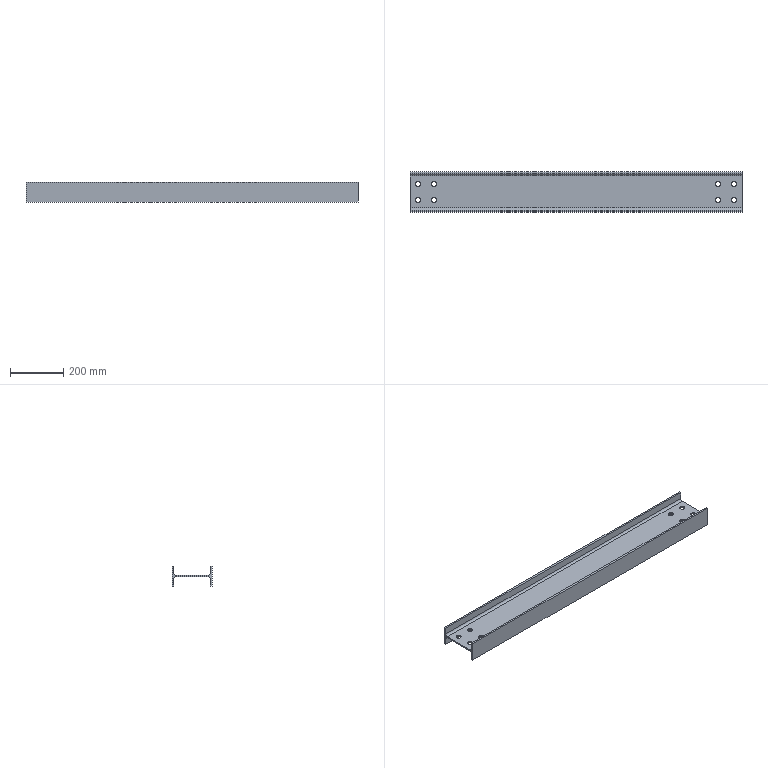Part | STEP file | 粉仓辅梁14主体_Default<As Machined> | 1 solid | 34 faces | box 1245 x 150 x 75 mm | volume 2210907 mm3 | cylinder 20 | plane 14 | commonest cylinder face diameters 19 x16 16 x4